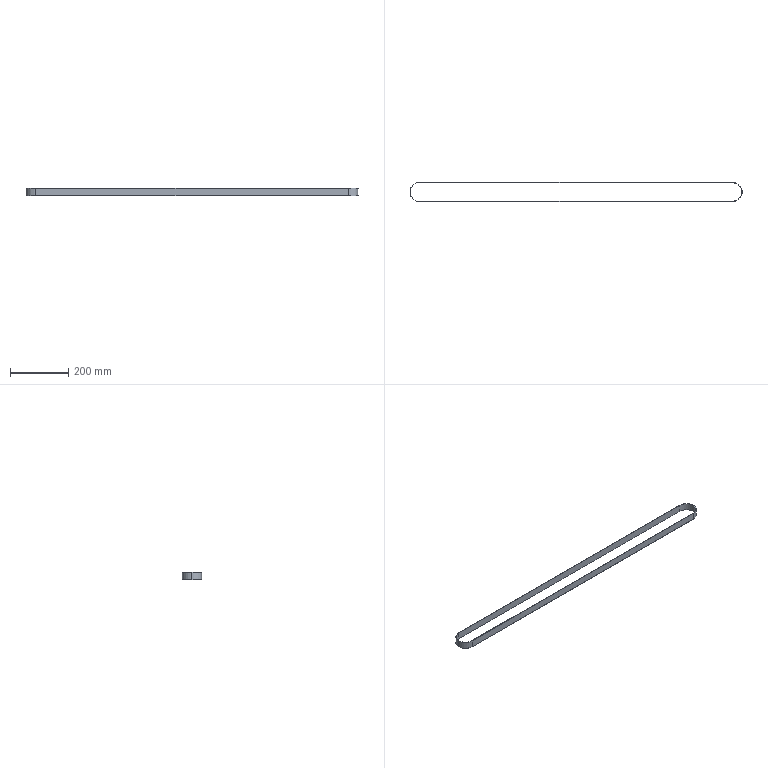Part | STEP file | Timing belt S5M-width 25-length 2350 (C-HTBN2350S5M-250, steel wire core) | 1 solid | 12 faces | box 1142 x 66.7 x 25 mm | volume 88306 mm3 | cylinder 6 | plane 6 | commonest cylinder face diameters 63.7 x3 66.7 x3
STEP:
#1=CARTESIAN_POINT('',(0.,0.,0.));
#2=DIRECTION('',(0.,0.,1.));
#3=DIRECTION('',(1.,0.,0.));
#4=AXIS2_PLACEMENT_3D('',#1,#2,#3);
#5=CARTESIAN_POINT('',(-537.5,31.85,12.5));
#6=VERTEX_POINT('',#5);
#7=CARTESIAN_POINT('',(-537.5,31.85,-12.5));
#8=VERTEX_POINT('',#7);
#9=CARTESIAN_POINT('',(-537.5,31.85,12.5));
#10=DIRECTION('',(0.,0.,-1.));
#11=VECTOR('',#10,1.);
#12=LINE('',#9,#11);
#13=CARTESIAN_POINT('',(-537.5,0.,12.5));
#14=DIRECTION('',(0.,0.,-1.));
#15=DIRECTION('',(-1.,0.,0.));
#16=AXIS2_PLACEMENT_3D('',#13,#14,#15);
#17=CYLINDRICAL_SURFACE('',#16,31.85);
#18=CARTESIAN_POINT('',(1.571,0.));
#19=DIRECTION('',(0.,1.));
#20=VECTOR('',#19,1.);
#21=LINE('',#18,#20);
#22=(GEOMETRIC_REPRESENTATION_CONTEXT(2)PARAMETRIC_REPRESENTATION_CONTEXT()REPRESENTATION_CONTEXT('',''));
#23=DEFINITIONAL_REPRESENTATION('',(#21),#22);
#24=PCURVE('',#17,#23);
#25=CARTESIAN_POINT('',(-537.5,31.85,12.5));
#26=DIRECTION('',(0.,-1.,0.));
#27=DIRECTION('',(0.,0.,-1.));
#28=AXIS2_PLACEMENT_3D('',#25,#26,#27);
#29=PLANE('',#28);
#30=CARTESIAN_POINT('',(0.,0.));
#31=DIRECTION('',(1.,0.));
#32=VECTOR('',#31,1.);
#33=LINE('',#30,#32);
#34=(GEOMETRIC_REPRESENTATION_CONTEXT(2)PARAMETRIC_REPRESENTATION_CONTEXT()REPRESENTATION_CONTEXT('',''));
#35=DEFINITIONAL_REPRESENTATION('',(#33),#34);
#36=PCURVE('',#29,#35);
#37=SURFACE_CURVE('',#12,(#24,#36),.PCURVE_S1.);
#38=EDGE_CURVE('',#6,#8,#37,.T.);
#39=ORIENTED_EDGE('',*,*,#38,.T.);
#40=CARTESIAN_POINT('',(-569.35,0.,-12.5));
#41=VERTEX_POINT('',#40);
#42=CARTESIAN_POINT('',(-537.5,0.,-12.5));
#43=DIRECTION('',(0.,0.,1.));
#44=DIRECTION('',(1.,0.,0.));
#45=AXIS2_PLACEMENT_3D('',#42,#43,#44);
#46=CIRCLE('',#45,31.85);
#47=CARTESIAN_POINT('',(3.142,25.));
#48=DIRECTION('',(-1.,0.));
#49=VECTOR('',#48,1.);
#50=LINE('',#47,#49);
#51=(GEOMETRIC_REPRESENTATION_CONTEXT(2)PARAMETRIC_REPRESENTATION_CONTEXT()REPRESENTATION_CONTEXT('',''));
#52=DEFINITIONAL_REPRESENTATION('',(#50),#51);
#53=PCURVE('',#17,#52);
#54=CARTESIAN_POINT('',(-537.5,0.,-12.5));
#55=DIRECTION('',(0.,0.,1.));
#56=DIRECTION('',(1.,0.,0.));
#57=AXIS2_PLACEMENT_3D('',#54,#55,#56);
#58=PLANE('',#57);
#59=CARTESIAN_POINT('',(0.,0.));
#60=DIRECTION('',(1.,0.));
#61=AXIS2_PLACEMENT_2D('',#59,#60);
#62=CIRCLE('',#61,31.85);
#63=(GEOMETRIC_REPRESENTATION_CONTEXT(2)PARAMETRIC_REPRESENTATION_CONTEXT()REPRESENTATION_CONTEXT('',''));
#64=DEFINITIONAL_REPRESENTATION('',(#62),#63);
#65=PCURVE('',#58,#64);
#66=SURFACE_CURVE('',#46,(#53,#65),.PCURVE_S1.);
#67=EDGE_CURVE('',#8,#41,#66,.T.);
#68=ORIENTED_EDGE('',*,*,#67,.T.);
#69=CARTESIAN_POINT('',(-569.35,0.,12.5));
#70=VERTEX_POINT('',#69);
#71=CARTESIAN_POINT('',(-569.35,0.,12.5));
#72=DIRECTION('',(0.,0.,-1.));
#73=VECTOR('',#72,1.);
#74=LINE('',#71,#73);
#75=CARTESIAN_POINT('',(0.,0.));
#76=DIRECTION('',(0.,1.));
#77=VECTOR('',#76,1.);
#78=LINE('',#75,#77);
#79=(GEOMETRIC_REPRESENTATION_CONTEXT(2)PARAMETRIC_REPRESENTATION_CONTEXT()REPRESENTATION_CONTEXT('',''));
#80=DEFINITIONAL_REPRESENTATION('',(#78),#79);
#81=PCURVE('',#17,#80);
#82=CARTESIAN_POINT('',(-537.5,0.,12.5));
#83=DIRECTION('',(0.,0.,-1.));
#84=DIRECTION('',(-1.,0.,0.));
#85=AXIS2_PLACEMENT_3D('',#82,#83,#84);
#86=CYLINDRICAL_SURFACE('',#85,31.85);
#87=CARTESIAN_POINT('',(6.283,0.));
#88=DIRECTION('',(0.,1.));
#89=VECTOR('',#88,1.);
#90=LINE('',#87,#89);
#91=(GEOMETRIC_REPRESENTATION_CONTEXT(2)PARAMETRIC_REPRESENTATION_CONTEXT()REPRESENTATION_CONTEXT('',''));
#92=DEFINITIONAL_REPRESENTATION('',(#90),#91);
#93=PCURVE('',#86,#92);
#94=SURFACE_CURVE('',#74,(#81,#93),.PCURVE_S1.);
#95=EDGE_CURVE('',#70,#41,#94,.T.);
#96=ORIENTED_EDGE('',*,*,#95,.F.);
#97=CARTESIAN_POINT('',(-537.5,0.,12.5));
#98=DIRECTION('',(0.,0.,1.));
#99=DIRECTION('',(1.,0.,0.));
#100=AXIS2_PLACEMENT_3D('',#97,#98,#99);
#101=CIRCLE('',#100,31.85);
#102=CARTESIAN_POINT('',(3.142,0.));
#103=DIRECTION('',(-1.,0.));
#104=VECTOR('',#103,1.);
#105=LINE('',#102,#104);
#106=(GEOMETRIC_REPRESENTATION_CONTEXT(2)PARAMETRIC_REPRESENTATION_CONTEXT()REPRESENTATION_CONTEXT('',''));
#107=DEFINITIONAL_REPRESENTATION('',(#105),#106);
#108=PCURVE('',#17,#107);
#109=CARTESIAN_POINT('',(-537.5,0.,12.5));
#110=DIRECTION('',(0.,0.,1.));
#111=DIRECTION('',(1.,0.,0.));
#112=AXIS2_PLACEMENT_3D('',#109,#110,#111);
#113=PLANE('',#112);
#114=CARTESIAN_POINT('',(0.,0.));
#115=DIRECTION('',(1.,0.));
#116=AXIS2_PLACEMENT_2D('',#114,#115);
#117=CIRCLE('',#116,31.85);
#118=(GEOMETRIC_REPRESENTATION_CONTEXT(2)PARAMETRIC_REPRESENTATION_CONTEXT()REPRESENTATION_CONTEXT('',''));
#119=DEFINITIONAL_REPRESENTATION('',(#117),#118);
#120=PCURVE('',#113,#119);
#121=SURFACE_CURVE('',#101,(#108,#120),.PCURVE_S1.);
#122=EDGE_CURVE('',#6,#70,#121,.T.);
#123=ORIENTED_EDGE('',*,*,#122,.F.);
#124=EDGE_LOOP('',(#39,#68,#96,#123));
#125=FACE_BOUND('',#124,.F.);
#126=ADVANCED_FACE('',(#125),#17,.F.);
#127=CARTESIAN_POINT('',(-570.85,0.,12.5));
#128=VERTEX_POINT('',#127);
#129=CARTESIAN_POINT('',(-537.5,-33.35,12.5));
#130=VERTEX_POINT('',#129);
#131=CARTESIAN_POINT('',(-537.5,0.,12.5));
#132=DIRECTION('',(0.,0.,1.));
#133=DIRECTION('',(1.,0.,0.));
#134=AXIS2_PLACEMENT_3D('',#131,#132,#133);
#135=CIRCLE('',#134,33.35);
#136=CARTESIAN_POINT('',(-537.5,0.,12.5));
#137=DIRECTION('',(0.,0.,-1.));
#138=DIRECTION('',(-1.,0.,0.));
#139=AXIS2_PLACEMENT_3D('',#136,#137,#138);
#140=CYLINDRICAL_SURFACE('',#139,33.35);
#141=CARTESIAN_POINT('',(9.425,0.));
#142=DIRECTION('',(-1.,0.));
#143=VECTOR('',#142,1.);
#144=LINE('',#141,#143);
#145=(GEOMETRIC_REPRESENTATION_CONTEXT(2)PARAMETRIC_REPRESENTATION_CONTEXT()REPRESENTATION_CONTEXT('',''));
#146=DEFINITIONAL_REPRESENTATION('',(#144),#145);
#147=PCURVE('',#140,#146);
#148=CARTESIAN_POINT('',(0.,0.));
#149=DIRECTION('',(1.,0.));
#150=AXIS2_PLACEMENT_2D('',#148,#149);
#151=CIRCLE('',#150,33.35);
#152=(GEOMETRIC_REPRESENTATION_CONTEXT(2)PARAMETRIC_REPRESENTATION_CONTEXT()REPRESENTATION_CONTEXT('',''));
#153=DEFINITIONAL_REPRESENTATION('',(#151),#152);
#154=PCURVE('',#113,#153);
#155=SURFACE_CURVE('',#135,(#147,#154),.PCURVE_S1.);
#156=EDGE_CURVE('',#128,#130,#155,.T.);
#157=ORIENTED_EDGE('',*,*,#156,.F.);
#158=CARTESIAN_POINT('',(-570.85,0.,-12.5));
#159=VERTEX_POINT('',#158);
#160=CARTESIAN_POINT('',(-570.85,0.,12.5));
#161=DIRECTION('',(0.,0.,-1.));
#162=VECTOR('',#161,1.);
#163=LINE('',#160,#162);
#164=CARTESIAN_POINT('',(6.283,0.));
#165=DIRECTION('',(0.,1.));
#166=VECTOR('',#165,1.);
#167=LINE('',#164,#166);
#168=(GEOMETRIC_REPRESENTATION_CONTEXT(2)PARAMETRIC_REPRESENTATION_CONTEXT()REPRESENTATION_CONTEXT('',''));
#169=DEFINITIONAL_REPRESENTATION('',(#167),#168);
#170=PCURVE('',#140,#169);
#171=CARTESIAN_POINT('',(-537.5,0.,12.5));
#172=DIRECTION('',(0.,0.,-1.));
#173=DIRECTION('',(-1.,0.,0.));
#174=AXIS2_PLACEMENT_3D('',#171,#172,#173);
#175=CYLINDRICAL_SURFACE('',#174,33.35);
#176=CARTESIAN_POINT('',(0.,0.));
#177=DIRECTION('',(0.,1.));
#178=VECTOR('',#177,1.);
#179=LINE('',#176,#178);
#180=(GEOMETRIC_REPRESENTATION_CONTEXT(2)PARAMETRIC_REPRESENTATION_CONTEXT()REPRESENTATION_CONTEXT('',''));
#181=DEFINITIONAL_REPRESENTATION('',(#179),#180);
#182=PCURVE('',#175,#181);
#183=SURFACE_CURVE('',#163,(#170,#182),.PCURVE_S1.);
#184=EDGE_CURVE('',#128,#159,#183,.T.);
#185=ORIENTED_EDGE('',*,*,#184,.T.);
#186=CARTESIAN_POINT('',(-537.5,-33.35,-12.5));
#187=VERTEX_POINT('',#186);
#188=CARTESIAN_POINT('',(-537.5,0.,-12.5));
#189=DIRECTION('',(0.,0.,1.));
#190=DIRECTION('',(1.,0.,0.));
#191=AXIS2_PLACEMENT_3D('',#188,#189,#190);
#192=CIRCLE('',#191,33.35);
#193=CARTESIAN_POINT('',(9.425,25.));
#194=DIRECTION('',(-1.,0.));
#195=VECTOR('',#194,1.);
#196=LINE('',#193,#195);
#197=(GEOMETRIC_REPRESENTATION_CONTEXT(2)PARAMETRIC_REPRESENTATION_CONTEXT()REPRESENTATION_CONTEXT('',''));
#198=DEFINITIONAL_REPRESENTATION('',(#196),#197);
#199=PCURVE('',#140,#198);
#200=CARTESIAN_POINT('',(0.,0.));
#201=DIRECTION('',(1.,0.));
#202=AXIS2_PLACEMENT_2D('',#200,#201);
#203=CIRCLE('',#202,33.35);
#204=(GEOMETRIC_REPRESENTATION_CONTEXT(2)PARAMETRIC_REPRESENTATION_CONTEXT()REPRESENTATION_CONTEXT('',''));
#205=DEFINITIONAL_REPRESENTATION('',(#203),#204);
#206=PCURVE('',#58,#205);
#207=SURFACE_CURVE('',#192,(#199,#206),.PCURVE_S1.);
#208=EDGE_CURVE('',#159,#187,#207,.T.);
#209=ORIENTED_EDGE('',*,*,#208,.T.);
#210=CARTESIAN_POINT('',(-537.5,-33.35,12.5));
#211=DIRECTION('',(0.,0.,-1.));
#212=VECTOR('',#211,1.);
#213=LINE('',#210,#212);
#214=CARTESIAN_POINT('',(4.712,0.));
#215=DIRECTION('',(0.,1.));
#216=VECTOR('',#215,1.);
#217=LINE('',#214,#216);
#218=(GEOMETRIC_REPRESENTATION_CONTEXT(2)PARAMETRIC_REPRESENTATION_CONTEXT()REPRESENTATION_CONTEXT('',''));
#219=DEFINITIONAL_REPRESENTATION('',(#217),#218);
#220=PCURVE('',#140,#219);
#221=CARTESIAN_POINT('',(-537.5,-33.35,12.5));
#222=DIRECTION('',(0.,1.,0.));
#223=DIRECTION('',(0.,0.,1.));
#224=AXIS2_PLACEMENT_3D('',#221,#222,#223);
#225=PLANE('',#224);
#226=CARTESIAN_POINT('',(0.,0.));
#227=DIRECTION('',(-1.,0.));
#228=VECTOR('',#227,1.);
#229=LINE('',#226,#228);
#230=(GEOMETRIC_REPRESENTATION_CONTEXT(2)PARAMETRIC_REPRESENTATION_CONTEXT()REPRESENTATION_CONTEXT('',''));
#231=DEFINITIONAL_REPRESENTATION('',(#229),#230);
#232=PCURVE('',#225,#231);
#233=SURFACE_CURVE('',#213,(#220,#232),.PCURVE_S1.);
#234=EDGE_CURVE('',#130,#187,#233,.T.);
#235=ORIENTED_EDGE('',*,*,#234,.F.);
#236=EDGE_LOOP('',(#157,#185,#209,#235));
#237=FACE_BOUND('',#236,.T.);
#238=ADVANCED_FACE('',(#237),#140,.T.);
#239=CARTESIAN_POINT('',(-537.5,33.35,12.5));
#240=VERTEX_POINT('',#239);
#241=CARTESIAN_POINT('',(-537.5,0.,12.5));
#242=DIRECTION('',(0.,0.,1.));
#243=DIRECTION('',(1.,0.,0.));
#244=AXIS2_PLACEMENT_3D('',#241,#242,#243);
#245=CIRCLE('',#244,33.35);
#246=CARTESIAN_POINT('',(0.,0.));
#247=DIRECTION('',(1.,0.));
#248=AXIS2_PLACEMENT_2D('',#246,#247);
#249=CIRCLE('',#248,33.35);
#250=(GEOMETRIC_REPRESENTATION_CONTEXT(2)PARAMETRIC_REPRESENTATION_CONTEXT()REPRESENTATION_CONTEXT('',''));
#251=DEFINITIONAL_REPRESENTATION('',(#249),#250);
#252=PCURVE('',#113,#251);
#253=CARTESIAN_POINT('',(3.142,0.));
#254=DIRECTION('',(-1.,0.));
#255=VECTOR('',#254,1.);
#256=LINE('',#253,#255);
#257=(GEOMETRIC_REPRESENTATION_CONTEXT(2)PARAMETRIC_REPRESENTATION_CONTEXT()REPRESENTATION_CONTEXT('',''));
#258=DEFINITIONAL_REPRESENTATION('',(#256),#257);
#259=PCURVE('',#175,#258);
#260=SURFACE_CURVE('',#245,(#252,#259),.PCURVE_S1.);
#261=EDGE_CURVE('',#240,#128,#260,.T.);
#262=ORIENTED_EDGE('',*,*,#261,.T.);
#263=ORIENTED_EDGE('',*,*,#156,.T.);
#264=CARTESIAN_POINT('',(537.5,-33.35,12.5));
#265=VERTEX_POINT('',#264);
#266=CARTESIAN_POINT('',(-537.5,-33.35,12.5));
#267=DIRECTION('',(1.,0.,0.));
#268=VECTOR('',#267,1.);
#269=LINE('',#266,#268);
#270=CARTESIAN_POINT('',(0.,-33.35));
#271=DIRECTION('',(1.,0.));
#272=VECTOR('',#271,1.);
#273=LINE('',#270,#272);
#274=(GEOMETRIC_REPRESENTATION_CONTEXT(2)PARAMETRIC_REPRESENTATION_CONTEXT()REPRESENTATION_CONTEXT('',''));
#275=DEFINITIONAL_REPRESENTATION('',(#273),#274);
#276=PCURVE('',#113,#275);
#277=CARTESIAN_POINT('',(0.,0.));
#278=DIRECTION('',(0.,1.));
#279=VECTOR('',#278,1.);
#280=LINE('',#277,#279);
#281=(GEOMETRIC_REPRESENTATION_CONTEXT(2)PARAMETRIC_REPRESENTATION_CONTEXT()REPRESENTATION_CONTEXT('',''));
#282=DEFINITIONAL_REPRESENTATION('',(#280),#281);
#283=PCURVE('',#225,#282);
#284=SURFACE_CURVE('',#269,(#276,#283),.PCURVE_S1.);
#285=EDGE_CURVE('',#130,#265,#284,.T.);
#286=ORIENTED_EDGE('',*,*,#285,.T.);
#287=CARTESIAN_POINT('',(537.5,33.35,12.5));
#288=VERTEX_POINT('',#287);
#289=CARTESIAN_POINT('',(537.5,0.,12.5));
#290=DIRECTION('',(0.,0.,1.));
#291=DIRECTION('',(1.,0.,0.));
#292=AXIS2_PLACEMENT_3D('',#289,#290,#291);
#293=CIRCLE('',#292,33.35);
#294=CARTESIAN_POINT('',(1075.,0.));
#295=DIRECTION('',(1.,0.));
#296=AXIS2_PLACEMENT_2D('',#294,#295);
#297=CIRCLE('',#296,33.35);
#298=(GEOMETRIC_REPRESENTATION_CONTEXT(2)PARAMETRIC_REPRESENTATION_CONTEXT()REPRESENTATION_CONTEXT('',''));
#299=DEFINITIONAL_REPRESENTATION('',(#297),#298);
#300=PCURVE('',#113,#299);
#301=CARTESIAN_POINT('',(537.5,0.,12.5));
#302=DIRECTION('',(0.,0.,-1.));
#303=DIRECTION('',(-1.,0.,0.));
#304=AXIS2_PLACEMENT_3D('',#301,#302,#303);
#305=CYLINDRICAL_SURFACE('',#304,33.35);
#306=CARTESIAN_POINT('',(9.425,0.));
#307=DIRECTION('',(-1.,0.));
#308=VECTOR('',#307,1.);
#309=LINE('',#306,#308);
#310=(GEOMETRIC_REPRESENTATION_CONTEXT(2)PARAMETRIC_REPRESENTATION_CONTEXT()REPRESENTATION_CONTEXT('',''));
#311=DEFINITIONAL_REPRESENTATION('',(#309),#310);
#312=PCURVE('',#305,#311);
#313=SURFACE_CURVE('',#293,(#300,#312),.PCURVE_S1.);
#314=EDGE_CURVE('',#265,#288,#313,.T.);
#315=ORIENTED_EDGE('',*,*,#314,.T.);
#316=CARTESIAN_POINT('',(-537.5,33.35,12.5));
#317=DIRECTION('',(-1.,0.,0.));
#318=VECTOR('',#317,1.);
#319=LINE('',#316,#318);
#320=CARTESIAN_POINT('',(0.,33.35));
#321=DIRECTION('',(-1.,0.));
#322=VECTOR('',#321,1.);
#323=LINE('',#320,#322);
#324=(GEOMETRIC_REPRESENTATION_CONTEXT(2)PARAMETRIC_REPRESENTATION_CONTEXT()REPRESENTATION_CONTEXT('',''));
#325=DEFINITIONAL_REPRESENTATION('',(#323),#324);
#326=PCURVE('',#113,#325);
#327=CARTESIAN_POINT('',(-537.5,33.35,12.5));
#328=DIRECTION('',(0.,-1.,0.));
#329=DIRECTION('',(0.,0.,-1.));
#330=AXIS2_PLACEMENT_3D('',#327,#328,#329);
#331=PLANE('',#330);
#332=CARTESIAN_POINT('',(0.,0.));
#333=DIRECTION('',(0.,-1.));
#334=VECTOR('',#333,1.);
#335=LINE('',#332,#334);
#336=(GEOMETRIC_REPRESENTATION_CONTEXT(2)PARAMETRIC_REPRESENTATION_CONTEXT()REPRESENTATION_CONTEXT('',''));
#337=DEFINITIONAL_REPRESENTATION('',(#335),#336);
#338=PCURVE('',#331,#337);
#339=SURFACE_CURVE('',#319,(#326,#338),.PCURVE_S1.);
#340=EDGE_CURVE('',#288,#240,#339,.T.);
#341=ORIENTED_EDGE('',*,*,#340,.T.);
#342=EDGE_LOOP('',(#262,#263,#286,#315,#341));
#343=FACE_BOUND('',#342,.T.);
#344=CARTESIAN_POINT('',(-537.5,-31.85,12.5));
#345=VERTEX_POINT('',#344);
#346=CARTESIAN_POINT('',(537.5,-31.85,12.5));
#347=VERTEX_POINT('',#346);
#348=CARTESIAN_POINT('',(-537.5,-31.85,12.5));
#349=DIRECTION('',(1.,0.,0.));
#350=VECTOR('',#349,1.);
#351=LINE('',#348,#350);
#352=CARTESIAN_POINT('',(0.,-31.85));
#353=DIRECTION('',(1.,0.));
#354=VECTOR('',#353,1.);
#355=LINE('',#352,#354);
#356=(GEOMETRIC_REPRESENTATION_CONTEXT(2)PARAMETRIC_REPRESENTATION_CONTEXT()REPRESENTATION_CONTEXT('',''));
#357=DEFINITIONAL_REPRESENTATION('',(#355),#356);
#358=PCURVE('',#113,#357);
#359=CARTESIAN_POINT('',(-537.5,-31.85,12.5));
#360=DIRECTION('',(0.,1.,0.));
#361=DIRECTION('',(0.,0.,1.));
#362=AXIS2_PLACEMENT_3D('',#359,#360,#361);
#363=PLANE('',#362);
#364=CARTESIAN_POINT('',(0.,0.));
#365=DIRECTION('',(0.,1.));
#366=VECTOR('',#365,1.);
#367=LINE('',#364,#366);
#368=(GEOMETRIC_REPRESENTATION_CONTEXT(2)PARAMETRIC_REPRESENTATION_CONTEXT()REPRESENTATION_CONTEXT('',''));
#369=DEFINITIONAL_REPRESENTATION('',(#367),#368);
#370=PCURVE('',#363,#369);
#371=SURFACE_CURVE('',#351,(#358,#370),.PCURVE_S1.);
#372=EDGE_CURVE('',#345,#347,#371,.T.);
#373=ORIENTED_EDGE('',*,*,#372,.F.);
#374=CARTESIAN_POINT('',(-537.5,0.,12.5));
#375=DIRECTION('',(0.,0.,1.));
#376=DIRECTION('',(1.,0.,0.));
#377=AXIS2_PLACEMENT_3D('',#374,#375,#376);
#378=CIRCLE('',#377,31.85);
#379=CARTESIAN_POINT('',(0.,0.));
#380=DIRECTION('',(1.,0.));
#381=AXIS2_PLACEMENT_2D('',#379,#380);
#382=CIRCLE('',#381,31.85);
#383=(GEOMETRIC_REPRESENTATION_CONTEXT(2)PARAMETRIC_REPRESENTATION_CONTEXT()REPRESENTATION_CONTEXT('',''));
#384=DEFINITIONAL_REPRESENTATION('',(#382),#383);
#385=PCURVE('',#113,#384);
#386=CARTESIAN_POINT('',(9.425,0.));
#387=DIRECTION('',(-1.,0.));
#388=VECTOR('',#387,1.);
#389=LINE('',#386,#388);
#390=(GEOMETRIC_REPRESENTATION_CONTEXT(2)PARAMETRIC_REPRESENTATION_CONTEXT()REPRESENTATION_CONTEXT('',''));
#391=DEFINITIONAL_REPRESENTATION('',(#389),#390);
#392=PCURVE('',#86,#391);
#393=SURFACE_CURVE('',#378,(#385,#392),.PCURVE_S1.);
#394=EDGE_CURVE('',#70,#345,#393,.T.);
#395=ORIENTED_EDGE('',*,*,#394,.F.);
#396=ORIENTED_EDGE('',*,*,#122,.F.);
#397=CARTESIAN_POINT('',(537.5,31.85,12.5));
#398=VERTEX_POINT('',#397);
#399=CARTESIAN_POINT('',(-537.5,31.85,12.5));
#400=DIRECTION('',(-1.,0.,0.));
#401=VECTOR('',#400,1.);
#402=LINE('',#399,#401);
#403=CARTESIAN_POINT('',(0.,31.85));
#404=DIRECTION('',(-1.,0.));
#405=VECTOR('',#404,1.);
#406=LINE('',#403,#405);
#407=(GEOMETRIC_REPRESENTATION_CONTEXT(2)PARAMETRIC_REPRESENTATION_CONTEXT()REPRESENTATION_CONTEXT('',''));
#408=DEFINITIONAL_REPRESENTATION('',(#406),#407);
#409=PCURVE('',#113,#408);
#410=CARTESIAN_POINT('',(0.,0.));
#411=DIRECTION('',(0.,-1.));
#412=VECTOR('',#411,1.);
#413=LINE('',#410,#412);
#414=(GEOMETRIC_REPRESENTATION_CONTEXT(2)PARAMETRIC_REPRESENTATION_CONTEXT()REPRESENTATION_CONTEXT('',''));
#415=DEFINITIONAL_REPRESENTATION('',(#413),#414);
#416=PCURVE('',#29,#415);
#417=SURFACE_CURVE('',#402,(#409,#416),.PCURVE_S1.);
#418=EDGE_CURVE('',#398,#6,#417,.T.);
#419=ORIENTED_EDGE('',*,*,#418,.F.);
#420=CARTESIAN_POINT('',(537.5,0.,12.5));
#421=DIRECTION('',(0.,0.,1.));
#422=DIRECTION('',(1.,0.,0.));
#423=AXIS2_PLACEMENT_3D('',#420,#421,#422);
#424=CIRCLE('',#423,31.85);
#425=CARTESIAN_POINT('',(1075.,0.));
#426=DIRECTION('',(1.,0.));
#427=AXIS2_PLACEMENT_2D('',#425,#426);
#428=CIRCLE('',#427,31.85);
#429=(GEOMETRIC_REPRESENTATION_CONTEXT(2)PARAMETRIC_REPRESENTATION_CONTEXT()REPRESENTATION_CONTEXT('',''));
#430=DEFINITIONAL_REPRESENTATION('',(#428),#429);
#431=PCURVE('',#113,#430);
#432=CARTESIAN_POINT('',(537.5,0.,12.5));
#433=DIRECTION('',(0.,0.,-1.));
#434=DIRECTION('',(-1.,0.,0.));
#435=AXIS2_PLACEMENT_3D('',#432,#433,#434);
#436=CYLINDRICAL_SURFACE('',#435,31.85);
#437=CARTESIAN_POINT('',(9.425,0.));
#438=DIRECTION('',(-1.,0.));
#439=VECTOR('',#438,1.);
#440=LINE('',#437,#439);
#441=(GEOMETRIC_REPRESENTATION_CONTEXT(2)PARAMETRIC_REPRESENTATION_CONTEXT()REPRESENTATION_CONTEXT('',''));
#442=DEFINITIONAL_REPRESENTATION('',(#440),#441);
#443=PCURVE('',#436,#442);
#444=SURFACE_CURVE('',#424,(#431,#443),.PCURVE_S1.);
#445=EDGE_CURVE('',#347,#398,#444,.T.);
#446=ORIENTED_EDGE('',*,*,#445,.F.);
#447=EDGE_LOOP('',(#373,#395,#396,#419,#446));
#448=FACE_BOUND('',#447,.T.);
#449=ADVANCED_FACE('',(#343,#448),#113,.T.);
#450=CARTESIAN_POINT('',(-537.5,33.35,-12.5));
#451=VERTEX_POINT('',#450);
#452=CARTESIAN_POINT('',(-537.5,0.,-12.5));
#453=DIRECTION('',(0.,0.,1.));
#454=DIRECTION('',(1.,0.,0.));
#455=AXIS2_PLACEMENT_3D('',#452,#453,#454);
#456=CIRCLE('',#455,33.35);
#457=CARTESIAN_POINT('',(0.,0.));
#458=DIRECTION('',(1.,0.));
#459=AXIS2_PLACEMENT_2D('',#457,#458);
#460=CIRCLE('',#459,33.35);
#461=(GEOMETRIC_REPRESENTATION_CONTEXT(2)PARAMETRIC_REPRESENTATION_CONTEXT()REPRESENTATION_CONTEXT('',''));
#462=DEFINITIONAL_REPRESENTATION('',(#460),#461);
#463=PCURVE('',#58,#462);
#464=CARTESIAN_POINT('',(3.142,25.));
#465=DIRECTION('',(-1.,0.));
#466=VECTOR('',#465,1.);
#467=LINE('',#464,#466);
#468=(GEOMETRIC_REPRESENTATION_CONTEXT(2)PARAMETRIC_REPRESENTATION_CONTEXT()REPRESENTATION_CONTEXT('',''));
#469=DEFINITIONAL_REPRESENTATION('',(#467),#468);
#470=PCURVE('',#175,#469);
#471=SURFACE_CURVE('',#456,(#463,#470),.PCURVE_S1.);
#472=EDGE_CURVE('',#451,#159,#471,.T.);
#473=ORIENTED_EDGE('',*,*,#472,.F.);
#474=CARTESIAN_POINT('',(537.5,33.35,-12.5));
#475=VERTEX_POINT('',#474);
#476=CARTESIAN_POINT('',(-537.5,33.35,-12.5));
#477=DIRECTION('',(-1.,0.,0.));
#478=VECTOR('',#477,1.);
#479=LINE('',#476,#478);
#480=CARTESIAN_POINT('',(0.,33.35));
#481=DIRECTION('',(-1.,0.));
#482=VECTOR('',#481,1.);
#483=LINE('',#480,#482);
#484=(GEOMETRIC_REPRESENTATION_CONTEXT(2)PARAMETRIC_REPRESENTATION_CONTEXT()REPRESENTATION_CONTEXT('',''));
#485=DEFINITIONAL_REPRESENTATION('',(#483),#484);
#486=PCURVE('',#58,#485);
#487=CARTESIAN_POINT('',(25.,0.));
#488=DIRECTION('',(0.,-1.));
#489=VECTOR('',#488,1.);
#490=LINE('',#487,#489);
#491=(GEOMETRIC_REPRESENTATION_CONTEXT(2)PARAMETRIC_REPRESENTATION_CONTEXT()REPRESENTATION_CONTEXT('',''));
#492=DEFINITIONAL_REPRESENTATION('',(#490),#491);
#493=PCURVE('',#331,#492);
#494=SURFACE_CURVE('',#479,(#486,#493),.PCURVE_S1.);
#495=EDGE_CURVE('',#475,#451,#494,.T.);
#496=ORIENTED_EDGE('',*,*,#495,.F.);
#497=CARTESIAN_POINT('',(537.5,-33.35,-12.5));
#498=VERTEX_POINT('',#497);
#499=CARTESIAN_POINT('',(537.5,0.,-12.5));
#500=DIRECTION('',(0.,0.,1.));
#501=DIRECTION('',(1.,0.,0.));
#502=AXIS2_PLACEMENT_3D('',#499,#500,#501);
#503=CIRCLE('',#502,33.35);
#504=CARTESIAN_POINT('',(1075.,0.));
#505=DIRECTION('',(1.,0.));
#506=AXIS2_PLACEMENT_2D('',#504,#505);
#507=CIRCLE('',#506,33.35);
#508=(GEOMETRIC_REPRESENTATION_CONTEXT(2)PARAMETRIC_REPRESENTATION_CONTEXT()REPRESENTATION_CONTEXT('',''));
#509=DEFINITIONAL_REPRESENTATION('',(#507),#508);
#510=PCURVE('',#58,#509);
#511=CARTESIAN_POINT('',(9.425,25.));
#512=DIRECTION('',(-1.,0.));
#513=VECTOR('',#512,1.);
#514=LINE('',#511,#513);
#515=(GEOMETRIC_REPRESENTATION_CONTEXT(2)PARAMETRIC_REPRESENTATION_CONTEXT()REPRESENTATION_CONTEXT('',''));
#516=DEFINITIONAL_REPRESENTATION('',(#514),#515);
#517=PCURVE('',#305,#516);
#518=SURFACE_CURVE('',#503,(#510,#517),.PCURVE_S1.);
#519=EDGE_CURVE('',#498,#475,#518,.T.);
#520=ORIENTED_EDGE('',*,*,#519,.F.);
#521=CARTESIAN_POINT('',(-537.5,-33.35,-12.5));
#522=DIRECTION('',(1.,0.,0.));
#523=VECTOR('',#522,1.);
#524=LINE('',#521,#523);
#525=CARTESIAN_POINT('',(0.,-33.35));
#526=DIRECTION('',(1.,0.));
#527=VECTOR('',#526,1.);
#528=LINE('',#525,#527);
#529=(GEOMETRIC_REPRESENTATION_CONTEXT(2)PARAMETRIC_REPRESENTATION_CONTEXT()REPRESENTATION_CONTEXT('',''));
#530=DEFINITIONAL_REPRESENTATION('',(#528),#529);
#531=PCURVE('',#58,#530);
#532=CARTESIAN_POINT('',(-25.,0.));
#533=DIRECTION('',(0.,1.));
#534=VECTOR('',#533,1.);
#535=LINE('',#532,#534);
#536=(GEOMETRIC_REPRESENTATION_CONTEXT(2)PARAMETRIC_REPRESENTATION_CONTEXT()REPRESENTATION_CONTEXT('',''));
#537=DEFINITIONAL_REPRESENTATION('',(#535),#536);
#538=PCURVE('',#225,#537);
#539=SURFACE_CURVE('',#524,(#531,#538),.PCURVE_S1.);
#540=EDGE_CURVE('',#187,#498,#539,.T.);
#541=ORIENTED_EDGE('',*,*,#540,.F.);
#542=ORIENTED_EDGE('',*,*,#208,.F.);
#543=EDGE_LOOP('',(#473,#496,#520,#541,#542));
#544=FACE_BOUND('',#543,.T.);
#545=ORIENTED_EDGE('',*,*,#67,.T.);
#546=CARTESIAN_POINT('',(-537.5,-31.85,-12.5));
#547=VERTEX_POINT('',#546);
#548=CARTESIAN_POINT('',(-537.5,0.,-12.5));
#549=DIRECTION('',(0.,0.,1.));
#550=DIRECTION('',(1.,0.,0.));
#551=AXIS2_PLACEMENT_3D('',#548,#549,#550);
#552=CIRCLE('',#551,31.85);
#553=CARTESIAN_POINT('',(0.,0.));
#554=DIRECTION('',(1.,0.));
#555=AXIS2_PLACEMENT_2D('',#553,#554);
#556=CIRCLE('',#555,31.85);
#557=(GEOMETRIC_REPRESENTATION_CONTEXT(2)PARAMETRIC_REPRESENTATION_CONTEXT()REPRESENTATION_CONTEXT('',''));
#558=DEFINITIONAL_REPRESENTATION('',(#556),#557);
#559=PCURVE('',#58,#558);
#560=CARTESIAN_POINT('',(9.425,25.));
#561=DIRECTION('',(-1.,0.));
#562=VECTOR('',#561,1.);
#563=LINE('',#560,#562);
#564=(GEOMETRIC_REPRESENTATION_CONTEXT(2)PARAMETRIC_REPRESENTATION_CONTEXT()REPRESENTATION_CONTEXT('',''));
#565=DEFINITIONAL_REPRESENTATION('',(#563),#564);
#566=PCURVE('',#86,#565);
#567=SURFACE_CURVE('',#552,(#559,#566),.PCURVE_S1.);
#568=EDGE_CURVE('',#41,#547,#567,.T.);
#569=ORIENTED_EDGE('',*,*,#568,.T.);
#570=CARTESIAN_POINT('',(537.5,-31.85,-12.5));
#571=VERTEX_POINT('',#570);
#572=CARTESIAN_POINT('',(-537.5,-31.85,-12.5));
#573=DIRECTION('',(1.,0.,0.));
#574=VECTOR('',#573,1.);
#575=LINE('',#572,#574);
#576=CARTESIAN_POINT('',(0.,-31.85));
#577=DIRECTION('',(1.,0.));
#578=VECTOR('',#577,1.);
#579=LINE('',#576,#578);
#580=(GEOMETRIC_REPRESENTATION_CONTEXT(2)PARAMETRIC_REPRESENTATION_CONTEXT()REPRESENTATION_CONTEXT('',''));
#581=DEFINITIONAL_REPRESENTATION('',(#579),#580);
#582=PCURVE('',#58,#581);
#583=CARTESIAN_POINT('',(-25.,0.));
#584=DIRECTION('',(0.,1.));
#585=VECTOR('',#584,1.);
#586=LINE('',#583,#585);
#587=(GEOMETRIC_REPRESENTATION_CONTEXT(2)PARAMETRIC_REPRESENTATION_CONTEXT()REPRESENTATION_CONTEXT('',''));
#588=DEFINITIONAL_REPRESENTATION('',(#586),#587);
#589=PCURVE('',#363,#588);
#590=SURFACE_CURVE('',#575,(#582,#589),.PCURVE_S1.);
#591=EDGE_CURVE('',#547,#571,#590,.T.);
#592=ORIENTED_EDGE('',*,*,#591,.T.);
#593=CARTESIAN_POINT('',(537.5,31.85,-12.5));
#594=VERTEX_POINT('',#593);
#595=CARTESIAN_POINT('',(537.5,0.,-12.5));
#596=DIRECTION('',(0.,0.,1.));
#597=DIRECTION('',(1.,0.,0.));
#598=AXIS2_PLACEMENT_3D('',#595,#596,#597);
#599=CIRCLE('',#598,31.85);
#600=CARTESIAN_POINT('',(1075.,0.));
#601=DIRECTION('',(1.,0.));
#602=AXIS2_PLACEMENT_2D('',#600,#601);
#603=CIRCLE('',#602,31.85);
#604=(GEOMETRIC_REPRESENTATION_CONTEXT(2)PARAMETRIC_REPRESENTATION_CONTEXT()REPRESENTATION_CONTEXT('',''));
#605=DEFINITIONAL_REPRESENTATION('',(#603),#604);
#606=PCURVE('',#58,#605);
#607=CARTESIAN_POINT('',(9.425,25.));
#608=DIRECTION('',(-1.,0.));
#609=VECTOR('',#608,1.);
#610=LINE('',#607,#609);
#611=(GEOMETRIC_REPRESENTATION_CONTEXT(2)PARAMETRIC_REPRESENTATION_CONTEXT()REPRESENTATION_CONTEXT('',''));
#612=DEFINITIONAL_REPRESENTATION('',(#610),#611);
#613=PCURVE('',#436,#612);
#614=SURFACE_CURVE('',#599,(#606,#613),.PCURVE_S1.);
#615=EDGE_CURVE('',#571,#594,#614,.T.);
#616=ORIENTED_EDGE('',*,*,#615,.T.);
#617=CARTESIAN_POINT('',(-537.5,31.85,-12.5));
#618=DIRECTION('',(-1.,0.,0.));
#619=VECTOR('',#618,1.);
#620=LINE('',#617,#619);
#621=CARTESIAN_POINT('',(0.,31.85));
#622=DIRECTION('',(-1.,0.));
#623=VECTOR('',#622,1.);
#624=LINE('',#621,#623);
#625=(GEOMETRIC_REPRESENTATION_CONTEXT(2)PARAMETRIC_REPRESENTATION_CONTEXT()REPRESENTATION_CONTEXT('',''));
#626=DEFINITIONAL_REPRESENTATION('',(#624),#625);
#627=PCURVE('',#58,#626);
#628=CARTESIAN_POINT('',(25.,0.));
#629=DIRECTION('',(0.,-1.));
#630=VECTOR('',#629,1.);
#631=LINE('',#628,#630);
#632=(GEOMETRIC_REPRESENTATION_CONTEXT(2)PARAMETRIC_REPRESENTATION_CONTEXT()REPRESENTATION_CONTEXT('',''));
#633=DEFINITIONAL_REPRESENTATION('',(#631),#632);
#634=PCURVE('',#29,#633);
#635=SURFACE_CURVE('',#620,(#627,#634),.PCURVE_S1.);
#636=EDGE_CURVE('',#594,#8,#635,.T.);
#637=ORIENTED_EDGE('',*,*,#636,.T.);
#638=EDGE_LOOP('',(#545,#569,#592,#616,#637));
#639=FACE_BOUND('',#638,.T.);
#640=ADVANCED_FACE('',(#544,#639),#58,.F.);
#641=ORIENTED_EDGE('',*,*,#184,.F.);
#642=ORIENTED_EDGE('',*,*,#261,.F.);
#643=CARTESIAN_POINT('',(-537.5,33.35,12.5));
#644=DIRECTION('',(0.,0.,-1.));
#645=VECTOR('',#644,1.);
#646=LINE('',#643,#645);
#647=CARTESIAN_POINT('',(1.571,0.));
#648=DIRECTION('',(0.,1.));
#649=VECTOR('',#648,1.);
#650=LINE('',#647,#649);
#651=(GEOMETRIC_REPRESENTATION_CONTEXT(2)PARAMETRIC_REPRESENTATION_CONTEXT()REPRESENTATION_CONTEXT('',''));
#652=DEFINITIONAL_REPRESENTATION('',(#650),#651);
#653=PCURVE('',#175,#652);
#654=CARTESIAN_POINT('',(0.,0.));
#655=DIRECTION('',(1.,0.));
#656=VECTOR('',#655,1.);
#657=LINE('',#654,#656);
#658=(GEOMETRIC_REPRESENTATION_CONTEXT(2)PARAMETRIC_REPRESENTATION_CONTEXT()REPRESENTATION_CONTEXT('',''));
#659=DEFINITIONAL_REPRESENTATION('',(#657),#658);
#660=PCURVE('',#331,#659);
#661=SURFACE_CURVE('',#646,(#653,#660),.PCURVE_S1.);
#662=EDGE_CURVE('',#240,#451,#661,.T.);
#663=ORIENTED_EDGE('',*,*,#662,.T.);
#664=ORIENTED_EDGE('',*,*,#472,.T.);
#665=EDGE_LOOP('',(#641,#642,#663,#664));
#666=FACE_BOUND('',#665,.T.);
#667=ADVANCED_FACE('',(#666),#175,.T.);
#668=ORIENTED_EDGE('',*,*,#540,.T.);
#669=CARTESIAN_POINT('',(537.5,-33.35,12.5));
#670=DIRECTION('',(0.,0.,-1.));
#671=VECTOR('',#670,1.);
#672=LINE('',#669,#671);
#673=CARTESIAN_POINT('',(0.,1075.));
#674=DIRECTION('',(-1.,0.));
#675=VECTOR('',#674,1.);
#676=LINE('',#673,#675);
#677=(GEOMETRIC_REPRESENTATION_CONTEXT(2)PARAMETRIC_REPRESENTATION_CONTEXT()REPRESENTATION_CONTEXT('',''));
#678=DEFINITIONAL_REPRESENTATION('',(#676),#677);
#679=PCURVE('',#225,#678);
#680=CARTESIAN_POINT('',(4.712,0.));
#681=DIRECTION('',(0.,1.));
#682=VECTOR('',#681,1.);
#683=LINE('',#680,#682);
#684=(GEOMETRIC_REPRESENTATION_CONTEXT(2)PARAMETRIC_REPRESENTATION_CONTEXT()REPRESENTATION_CONTEXT('',''));
#685=DEFINITIONAL_REPRESENTATION('',(#683),#684);
#686=PCURVE('',#305,#685);
#687=SURFACE_CURVE('',#672,(#679,#686),.PCURVE_S1.);
#688=EDGE_CURVE('',#265,#498,#687,.T.);
#689=ORIENTED_EDGE('',*,*,#688,.F.);
#690=ORIENTED_EDGE('',*,*,#285,.F.);
#691=ORIENTED_EDGE('',*,*,#234,.T.);
#692=EDGE_LOOP('',(#668,#689,#690,#691));
#693=FACE_BOUND('',#692,.T.);
#694=ADVANCED_FACE('',(#693),#225,.F.);
#695=ORIENTED_EDGE('',*,*,#519,.T.);
#696=CARTESIAN_POINT('',(537.5,33.35,12.5));
#697=DIRECTION('',(0.,0.,-1.));
#698=VECTOR('',#697,1.);
#699=LINE('',#696,#698);
#700=CARTESIAN_POINT('',(1.571,0.));
#701=DIRECTION('',(0.,1.));
#702=VECTOR('',#701,1.);
#703=LINE('',#700,#702);
#704=(GEOMETRIC_REPRESENTATION_CONTEXT(2)PARAMETRIC_REPRESENTATION_CONTEXT()REPRESENTATION_CONTEXT('',''));
#705=DEFINITIONAL_REPRESENTATION('',(#703),#704);
#706=PCURVE('',#305,#705);
#707=CARTESIAN_POINT('',(0.,1075.));
#708=DIRECTION('',(1.,0.));
#709=VECTOR('',#708,1.);
#710=LINE('',#707,#709);
#711=(GEOMETRIC_REPRESENTATION_CONTEXT(2)PARAMETRIC_REPRESENTATION_CONTEXT()REPRESENTATION_CONTEXT('',''));
#712=DEFINITIONAL_REPRESENTATION('',(#710),#711);
#713=PCURVE('',#331,#712);
#714=SURFACE_CURVE('',#699,(#706,#713),.PCURVE_S1.);
#715=EDGE_CURVE('',#288,#475,#714,.T.);
#716=ORIENTED_EDGE('',*,*,#715,.F.);
#717=ORIENTED_EDGE('',*,*,#314,.F.);
#718=ORIENTED_EDGE('',*,*,#688,.T.);
#719=EDGE_LOOP('',(#695,#716,#717,#718));
#720=FACE_BOUND('',#719,.T.);
#721=ADVANCED_FACE('',(#720),#305,.T.);
#722=ORIENTED_EDGE('',*,*,#495,.T.);
#723=ORIENTED_EDGE('',*,*,#662,.F.);
#724=ORIENTED_EDGE('',*,*,#340,.F.);
#725=ORIENTED_EDGE('',*,*,#715,.T.);
#726=EDGE_LOOP('',(#722,#723,#724,#725));
#727=FACE_BOUND('',#726,.T.);
#728=ADVANCED_FACE('',(#727),#331,.F.);
#729=ORIENTED_EDGE('',*,*,#568,.T.);
#730=CARTESIAN_POINT('',(-537.5,-31.85,12.5));
#731=DIRECTION('',(0.,0.,-1.));
#732=VECTOR('',#731,1.);
#733=LINE('',#730,#732);
#734=CARTESIAN_POINT('',(4.712,0.));
#735=DIRECTION('',(0.,1.));
#736=VECTOR('',#735,1.);
#737=LINE('',#734,#736);
#738=(GEOMETRIC_REPRESENTATION_CONTEXT(2)PARAMETRIC_REPRESENTATION_CONTEXT()REPRESENTATION_CONTEXT('',''));
#739=DEFINITIONAL_REPRESENTATION('',(#737),#738);
#740=PCURVE('',#86,#739);
#741=CARTESIAN_POINT('',(0.,0.));
#742=DIRECTION('',(-1.,0.));
#743=VECTOR('',#742,1.);
#744=LINE('',#741,#743);
#745=(GEOMETRIC_REPRESENTATION_CONTEXT(2)PARAMETRIC_REPRESENTATION_CONTEXT()REPRESENTATION_CONTEXT('',''));
#746=DEFINITIONAL_REPRESENTATION('',(#744),#745);
#747=PCURVE('',#363,#746);
#748=SURFACE_CURVE('',#733,(#740,#747),.PCURVE_S1.);
#749=EDGE_CURVE('',#345,#547,#748,.T.);
#750=ORIENTED_EDGE('',*,*,#749,.F.);
#751=ORIENTED_EDGE('',*,*,#394,.F.);
#752=ORIENTED_EDGE('',*,*,#95,.T.);
#753=EDGE_LOOP('',(#729,#750,#751,#752));
#754=FACE_BOUND('',#753,.F.);
#755=ADVANCED_FACE('',(#754),#86,.F.);
#756=ORIENTED_EDGE('',*,*,#591,.F.);
#757=ORIENTED_EDGE('',*,*,#749,.F.);
#758=ORIENTED_EDGE('',*,*,#372,.T.);
#759=CARTESIAN_POINT('',(537.5,-31.85,12.5));
#760=DIRECTION('',(0.,0.,-1.));
#761=VECTOR('',#760,1.);
#762=LINE('',#759,#761);
#763=CARTESIAN_POINT('',(0.,1075.));
#764=DIRECTION('',(-1.,0.));
#765=VECTOR('',#764,1.);
#766=LINE('',#763,#765);
#767=(GEOMETRIC_REPRESENTATION_CONTEXT(2)PARAMETRIC_REPRESENTATION_CONTEXT()REPRESENTATION_CONTEXT('',''));
#768=DEFINITIONAL_REPRESENTATION('',(#766),#767);
#769=PCURVE('',#363,#768);
#770=CARTESIAN_POINT('',(4.712,0.));
#771=DIRECTION('',(0.,1.));
#772=VECTOR('',#771,1.);
#773=LINE('',#770,#772);
#774=(GEOMETRIC_REPRESENTATION_CONTEXT(2)PARAMETRIC_REPRESENTATION_CONTEXT()REPRESENTATION_CONTEXT('',''));
#775=DEFINITIONAL_REPRESENTATION('',(#773),#774);
#776=PCURVE('',#436,#775);
#777=SURFACE_CURVE('',#762,(#769,#776),.PCURVE_S1.);
#778=EDGE_CURVE('',#347,#571,#777,.T.);
#779=ORIENTED_EDGE('',*,*,#778,.T.);
#780=EDGE_LOOP('',(#756,#757,#758,#779));
#781=FACE_BOUND('',#780,.T.);
#782=ADVANCED_FACE('',(#781),#363,.T.);
#783=CARTESIAN_POINT('',(537.5,31.85,12.5));
#784=DIRECTION('',(0.,0.,-1.));
#785=VECTOR('',#784,1.);
#786=LINE('',#783,#785);
#787=CARTESIAN_POINT('',(1.571,0.));
#788=DIRECTION('',(0.,1.));
#789=VECTOR('',#788,1.);
#790=LINE('',#787,#789);
#791=(GEOMETRIC_REPRESENTATION_CONTEXT(2)PARAMETRIC_REPRESENTATION_CONTEXT()REPRESENTATION_CONTEXT('',''));
#792=DEFINITIONAL_REPRESENTATION('',(#790),#791);
#793=PCURVE('',#436,#792);
#794=CARTESIAN_POINT('',(0.,1075.));
#795=DIRECTION('',(1.,0.));
#796=VECTOR('',#795,1.);
#797=LINE('',#794,#796);
#798=(GEOMETRIC_REPRESENTATION_CONTEXT(2)PARAMETRIC_REPRESENTATION_CONTEXT()REPRESENTATION_CONTEXT('',''));
#799=DEFINITIONAL_REPRESENTATION('',(#797),#798);
#800=PCURVE('',#29,#799);
#801=SURFACE_CURVE('',#786,(#793,#800),.PCURVE_S1.);
#802=EDGE_CURVE('',#398,#594,#801,.T.);
#803=ORIENTED_EDGE('',*,*,#802,.F.);
#804=ORIENTED_EDGE('',*,*,#445,.F.);
#805=ORIENTED_EDGE('',*,*,#778,.T.);
#806=ORIENTED_EDGE('',*,*,#615,.T.);
#807=EDGE_LOOP('',(#803,#804,#805,#806));
#808=FACE_BOUND('',#807,.F.);
#809=ADVANCED_FACE('',(#808),#436,.F.);
#810=ORIENTED_EDGE('',*,*,#636,.F.);
#811=ORIENTED_EDGE('',*,*,#802,.F.);
#812=ORIENTED_EDGE('',*,*,#418,.T.);
#813=ORIENTED_EDGE('',*,*,#38,.T.);
#814=EDGE_LOOP('',(#810,#811,#812,#813));
#815=FACE_BOUND('',#814,.T.);
#816=ADVANCED_FACE('',(#815),#29,.T.);
#817=CLOSED_SHELL('',(#126,#238,#449,#640,#667,#694,#721,#728,#755,#782,#809,#816));
#818=MANIFOLD_SOLID_BREP('',#817);
#819=(LENGTH_UNIT()NAMED_UNIT(*)SI_UNIT(.MILLI.,.METRE.));
#820=UNCERTAINTY_MEASURE_WITH_UNIT(LENGTH_MEASURE(0.0000001),#819,'','');
#821=(NAMED_UNIT(*)PLANE_ANGLE_UNIT()SI_UNIT($,.RADIAN.));
#822=(NAMED_UNIT(*)SI_UNIT($,.STERADIAN.)SOLID_ANGLE_UNIT());
#823=(GEOMETRIC_REPRESENTATION_CONTEXT(3)GLOBAL_UNCERTAINTY_ASSIGNED_CONTEXT((#820))GLOBAL_UNIT_ASSIGNED_CONTEXT((#819,#821,#822))REPRESENTATION_CONTEXT('',''));
#824=ADVANCED_BREP_SHAPE_REPRESENTATION('',(#4,#818),#823);